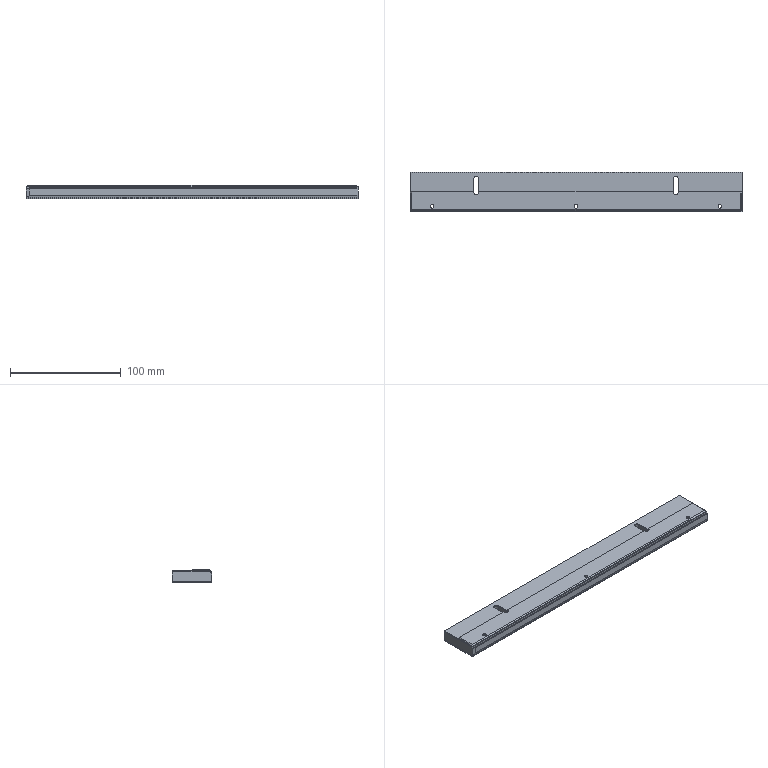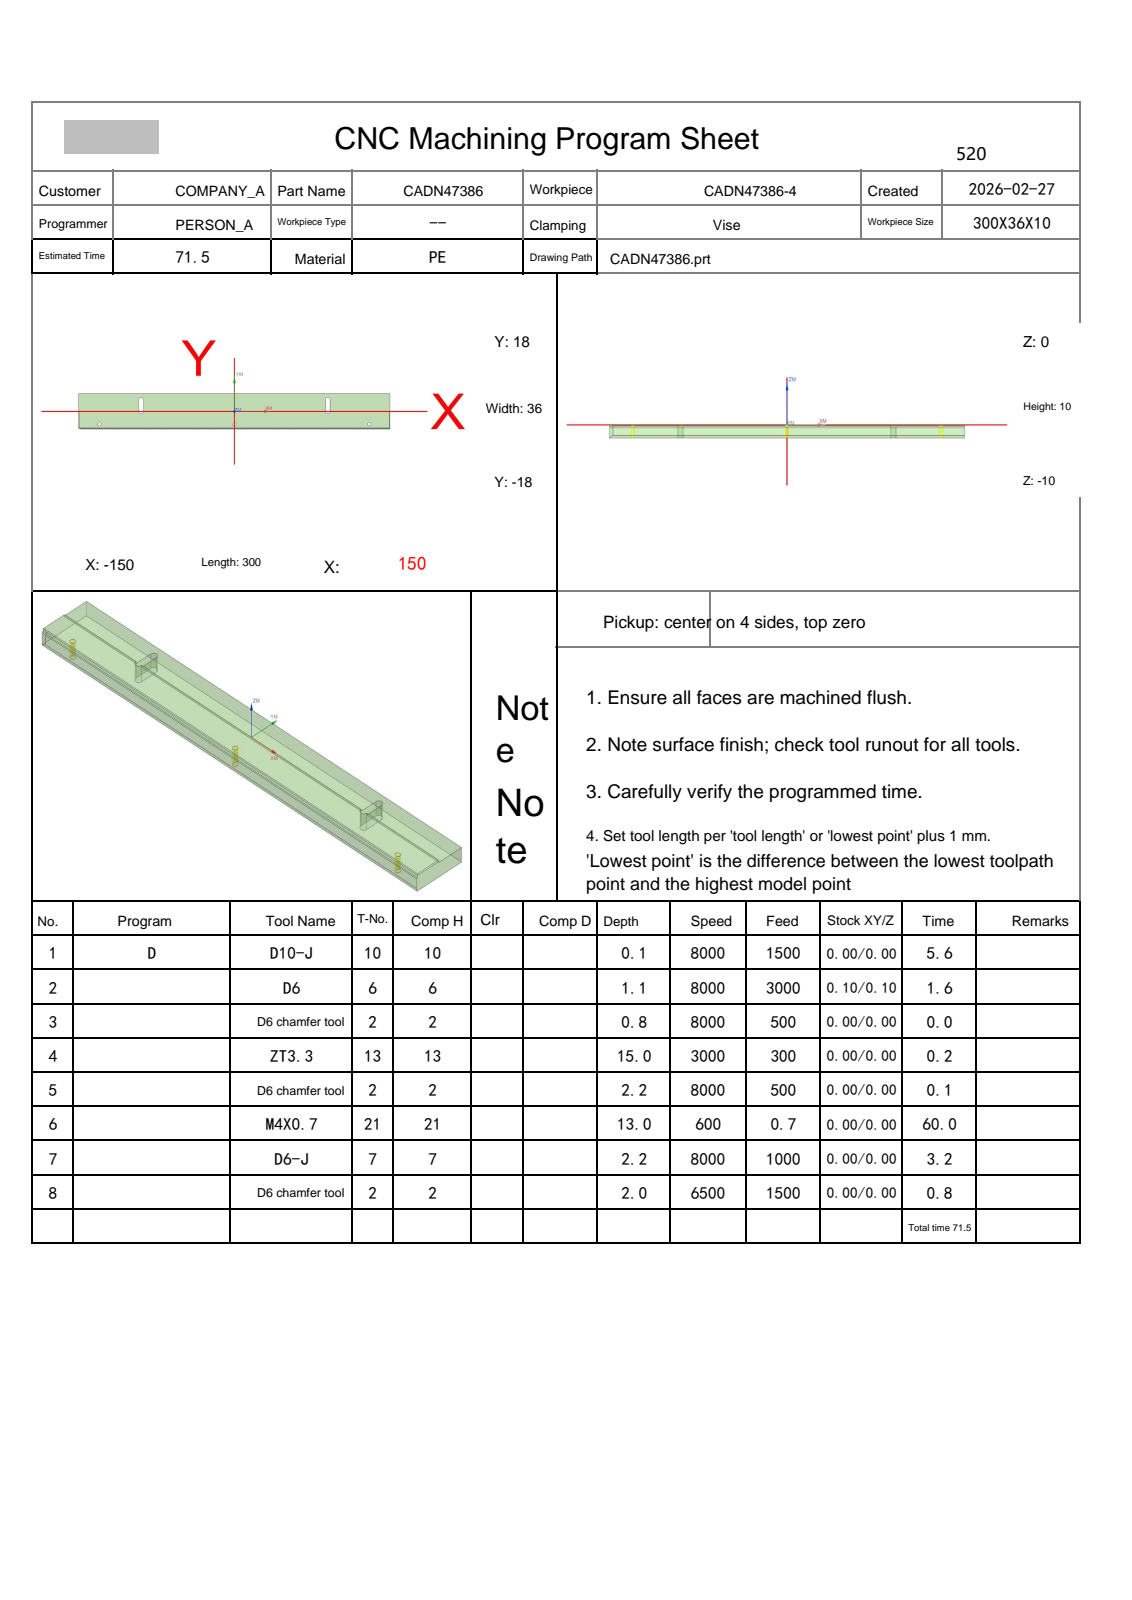NC program | NX | posted by the shop | part box 300 x 36 x 12 mm
Whole program:
%
O0001
(Machine time: 128.86 MIN)
(===Total Tool:6===)
(T10=D10-J  D=10.  R=0.   D-  H10 Z=0.    )
(T6=D6      D=6.   R=0.   D-  H06 Z=-1.1  )
(T2=D6 chamfer tool   D=6.   R=0.   D-  H02 Z=-2.17 )
(T13=ZT3.3  D=3.3  DR_a=118 D-  H13 Z=-15.  )
(T21=M4X0.7 D=3.3  DR_a=180 D-  H21 Z=-13.  )
(T7=D6-J    D=6.   R=0.   D7  H07 Z=-2.2  )
G80 G90 G17 G49 G40
G91 G28 Z0
M01
N1 T10 M06
(D10-J  D=10. R=0. H=10 ce=0.00 di=0.10)
G00 G90 G54 X-160. Y8.111 M03 S4500
G43 H10 Z30.
M08
Z2.55
G01 Z.55 F1500.
X-155. Y13.111
X-145.111 Y23.
X-135.222
X-155. Y3.222
Y-6.667
X-125.333 Y23.
X-115.444
X-155. Y-16.556
Y-23.
X-151.556
X-105.556 Y23.
X-95.667
X-141.667 Y-23.
X-131.778
X-85.778 Y23.
X-75.889
X-121.889 Y-23.
X-112.
X-66. Y23.
X-56.111
X-102.111 Y-23.
X-92.222
X-46.222 Y23.
X-36.333
X-82.333 Y-23.
X-72.444
X-26.444 Y23.
X-16.556
X-62.556 Y-23.
X-52.667
X-6.667 Y23.
X3.222
X-42.778 Y-23.
X-32.889
X13.111 Y23.
X23.
X-23. Y-23.
X-13.111
X32.889 Y23.
X42.778
X-3.222 Y-23.
X6.667
X52.667 Y23.
X62.556
X16.556 Y-23.
X26.444
X72.444 Y23.
X82.333
X36.333 Y-23.
X46.222
X92.222 Y23.
X102.111
X56.111 Y-23.
X66.
X112. Y23.
X121.889
X75.889 Y-23.
X85.778
X131.778 Y23.
X141.667
X95.667 Y-23.
X105.556
X151.556 Y23.
X155.
Y16.556
X115.444 Y-23.
X125.333
X155. Y6.667
Y-3.222
X135.222 Y-23.
X145.111
X155. Y-13.111
X160. Y-8.111
Z2.55
G00 Z4.
X-160. Y8.111
Z2.1
G01 Z.1
X-155. Y13.111
X-145.111 Y23.
X-135.222
X-155. Y3.222
Y-6.667
X-125.333 Y23.
X-115.444
X-155. Y-16.556
Y-23.
X-151.556
X-105.556 Y23.
X-95.667
X-141.667 Y-23.
X-131.778
X-85.778 Y23.
X-75.889
X-121.889 Y-23.
X-112.
X-66. Y23.
X-56.111
X-102.111 Y-23.
X-92.222
X-46.222 Y23.
X-36.333
X-82.333 Y-23.
X-72.444
X-26.444 Y23.
X-16.556
X-62.556 Y-23.
X-52.667
X-6.667 Y23.
X3.222
X-42.778 Y-23.
X-32.889
X13.111 Y23.
X23.
X-23. Y-23.
X-13.111
X32.889 Y23.
X42.778
X-3.222 Y-23.
X6.667
X52.667 Y23.
X62.556
X16.556 Y-23.
X26.444
X72.444 Y23.
X82.333
X36.333 Y-23.
X46.222
X92.222 Y23.
X102.111
X56.111 Y-23.
X66.
X112. Y23.
X121.889
X75.889 Y-23.
X85.778
X131.778 Y23.
X141.667
X95.667 Y-23.
X105.556
X151.556 Y23.
X155.
Y16.556
X115.444 Y-23.
X125.333
X155. Y6.667
Y-3.222
X135.222 Y-23.
X145.111
X155. Y-13.111
X160. Y-8.111
Z2.1
G00 Z30.
G00 G90 X133.111 Y35. M03 S8000
Z30.
Z2.
G01 Z0.0 F1000.
X145.111 Y23.
X155. Y13.111
Y3.222
X135.222 Y23.
X125.333
X155. Y-6.667
Y-16.556
X115.444 Y23.
X105.556
X151.556 Y-23.
X141.667
X95.667 Y23.
X85.778
X131.778 Y-23.
X121.889
X75.889 Y23.
X66.
X112. Y-23.
X102.111
X56.111 Y23.
X46.222
X92.222 Y-23.
X82.333
X36.333 Y23.
X26.444
X72.444 Y-23.
X62.556
X16.556 Y23.
X6.667
X52.667 Y-23.
X42.778
X-3.222 Y23.
X-13.111
X32.889 Y-23.
X23.
X-23. Y23.
X-32.889
X13.111 Y-23.
X3.222
X-42.778 Y23.
X-52.667
X-6.667 Y-23.
X-16.556
X-62.556 Y23.
X-72.444
X-26.444 Y-23.
X-36.333
X-82.333 Y23.
X-92.222
X-46.222 Y-23.
X-56.111
X-102.111 Y23.
X-112.
X-66. Y-23.
X-75.889
X-121.889 Y23.
X-131.778
X-85.778 Y-23.
X-95.667
X-141.667 Y23.
X-151.556
X-105.556 Y-23.
X-115.444
X-155. Y16.556
Y6.667
X-125.333 Y-23.
X-135.222
X-155. Y-3.222
Y-13.111
X-145.111 Y-23.
X-133.111 Y-35.
Z2.
G00 Z30.
G91 G28 Z0.0
M05
M09
G91 G28 Z0.0
M01
N2 T06 M06
(D6  D=6. R=0. H=06 ce=0.10 di=0.10)
G00 G90 G54 X-156. Y19.6 M03 S8000
G43 H06 Z11.
M08
Z1.133
G01 Z-.367 F3000.
X-152.94
X152.4
G02 X152.94 Y19.06 I0.0 J-.54
G01 Y17.2
G02 X152.34 Y16.6 I-.6 J0.0
G01 X-152.341
G03 X-152.94 Y16.001 I.001 J-.6
G01 Y12.699
G03 X-152.341 Y12.1 I.6 J.001
G01 X152.341
G02 X152.94 Y11.501 I-.001 J-.6
G01 Y8.199
G02 X152.341 Y7.6 I-.6 J.001
G01 X-152.427
G03 X-153.019 Y7.093 I.001 J-.6
G01 X-153.533 Y3.792
X-153.54 Y3.7
G03 X-152.94 Y3.1 I.6 J0.0
G01 X152.94
X156.
Z1.133
G00 X-156. Y19.6
Z.767
G01 Z-.733
X-152.94
X152.4
G02 X152.94 Y19.06 I0.0 J-.54
G01 Y17.2
G02 X152.34 Y16.6 I-.6 J0.0
G01 X-152.341
G03 X-152.94 Y16.001 I.001 J-.6
G01 Y12.699
G03 X-152.341 Y12.1 I.6 J.001
G01 X152.341
G02 X152.94 Y11.501 I-.001 J-.6
G01 Y8.199
G02 X152.341 Y7.6 I-.6 J.001
G01 X-152.427
G03 X-153.019 Y7.093 I.001 J-.6
G01 X-153.533 Y3.792
X-153.54 Y3.7
G03 X-152.94 Y3.1 I.6 J0.0
G01 X152.94
X156.1
Z.767
G00 X-156. Y19.6
Z.4
G01 Z-1.1
X-152.94
X152.4
G02 X152.94 Y19.06 I0.0 J-.54
G01 Y17.2
G02 X152.34 Y16.6 I-.6 J0.0
G01 X-152.341
G03 X-152.94 Y16.001 I.001 J-.6
G01 Y12.699
G03 X-152.341 Y12.1 I.6 J.001
G01 X152.341
G02 X152.94 Y11.501 I-.001 J-.6
G01 Y8.199
G02 X152.341 Y7.6 I-.6 J.001
G01 X-152.427
G03 X-153.019 Y7.093 I.001 J-.6
G01 X-153.533 Y3.792
X-153.54 Y3.7
G03 X-152.94 Y3.1 I.6 J0.0
G01 X152.94
X156.1
Z.4
G00 Z11.
G91 G28 Z0.0
M05
M09
G91 G28 Z0.0
M01
N3 T02 M06
(D6 chamfer tool  D=6. R=0. H=02 ce=0.00 di=0.10)
G00 G90 G54 X130. Y-13. M03 S8000
G43 H02 Z30.
M08
G98 G81 X130. Y-13. Z-.8 R1. F500.
X0.0
X-130.
G80
G00 Z30.
G91 G28 Z0.0
M05
M09
G91 G28 Z0.0
M01
N4 T13 M06
(ZT3.3 D=3.3 DR_a=118 H=13)
G00 G90 G54 X130. Y-13. M03 S3000
G43 H13 Z30.
M08
G98 G83 X130. Y-13. Z-15. R1. F300. Q2.
X0.0
X-130.
G80
G00 Z30.
G91 G28 Z0.0
M05
M09
G91 G28 Z0.0
M01
N5 T02 M06
(D6 chamfer tool  D=6. R=0. H=02 ce=0.00 di=0.10)
G00 G90 G54 X130. Y-13. M03 S8000
G43 H02 Z30.
M08
G98 G81 X130. Y-13. Z-2.171 R3. F500.
X0.0
X-130.
G80
G00 Z30.
G91 G28 Z0.0
M05
M09
G91 G28 Z0.0
M01
N6 T21 M06
(M4X0.7 D=3.3 DR_a=180 H=21)
G00 G90 G54 X130. Y-13. M03 S600
G43 H21 Z30.
M08
G95
G98 G84 X130. Y-13. Z-13. R1. F.7 Q4.
X0.0
X-130.
G80
G94
G00 Z30.
G91 G28 Z0.0
M05
M09
G91 G28 Z0.0
M01
N7 T07 M06
(D6-J  D=6. R=0. H=07 ce=0.40 di=0.00)
G00 G90 G54 X-1.2 Y22.2 M03 S8000
G43 H07 Z11.
M08
Z.3
G01 Z-1.2 F1000.
Y19.8
G03 X0.0 Y18.6 I1.2 J0.0
G01 X150.004
G02 X150.6 Y18.004 I-.004 J-.6
G01 Y3.996
G02 X150.004 Y3.4 I-.6 J.004
G01 X-150.004
G02 X-150.6 Y3.996 I.004 J.6
G01 Y18.004
G02 X-150.004 Y18.6 I.6 J-.004
G01 X1.252
G02 X1.675 Y18.425 I-.001 J-.6
G01 X4.325 Y15.775
G03 X4.748 Y15.6 I.424 J.425
G01 X147.004
G02 X147.6 Y15.004 I-.004 J-.6
G01 Y6.996
G02 X147.004 Y6.4 I-.6 J.004
G01 X-147.004
G02 X-147.6 Y6.996 I.004 J.6
G01 Y15.004
G02 X-147.004 Y15.6 I.6 J-.004
G01 X1.252
G02 X1.675 Y15.425 I-.001 J-.6
G01 X4.325 Y12.775
G03 X4.748 Y12.6 I.424 J.425
G01 X144.004
G02 X144.6 Y12.004 I-.004 J-.6
G01 Y9.996
G02 X144.004 Y9.4 I-.6 J.004
G01 X88.85
X-144.004
G02 X-144.6 Y9.996 I.004 J.6
G01 Y12.004
G02 X-144.004 Y12.6 I.6 J-.004
G01 X3.
X4.
G03 X5.2 Y13.8 I0.0 J1.2
G01 Z.3
G00 Z11.
G00 G90 X-154.2 Y4.399 M03 S8000
Z11.
Z-.2
G01 Z-1.2 F1000.
G41 D07
Y4.199
G03 X-153. Y3. I1.2 J.001
G01 X153.
G03 X154.2 Y4.199 I0.0 J1.2
G01 G40 Y4.399
Z-.2
G00 Z11.
G00 G90 X153.916 Y-21.226 M03 S8000
Z11.
Z.719
G01 Z-.781 F1000.
G41 D07
X153.9 Y-21.027
G03 X153.003 Y-20.2 I-.897 J-.073
G01 X-147.248
X-153.455 Y-19.165
X-153.603 Y-19.153
G03 X-153.9 Y-19.204 I0.0 J-.9
G01 G40 X-154.089 Y-19.27
Z.719
G00 Z11.
X153.916 Y-21.226
Z.01
G01 Z-1.49
G41 D07
X153.9 Y-21.027
G03 X153.003 Y-20.2 I-.897 J-.073
G01 X-147.248
X-153.455 Y-19.165
X-153.603 Y-19.153
G03 X-153.9 Y-19.204 I0.0 J-.9
G01 G40 X-154.089 Y-19.27
Z.01
G00 Z11.
X153.916 Y-21.226
Z-.7
G01 Z-2.2
G41 D07
X153.9 Y-21.027
G03 X153.003 Y-20.2 I-.897 J-.073
G01 X-147.248
X-153.455 Y-19.165
X-153.603 Y-19.153
G03 X-153.9 Y-19.204 I0.0 J-.9
G01 G40 X-154.089 Y-19.27
Z-.7
G00 Z11.
G91 G28 Z0.0
M05
M09
G91 G28 Z0.0
M01
N8 T02 M06
(D6 chamfer tool  D=6. R=0. H=02 ce=0.00 di=0.00)
G00 G90 G54 X-149.769 Y.528 M03 S6500
G43 H02 Z30.
M08
Z3.2
G01 Z-.8 F1500.
X-149.685 Y.571
X-149.5 Y.6
X-92.25
G02 X-91.65 Y0.0 I0.0 J-.6
G01 Y-.2
G03 X-90. Y-1.85 I1.65 J0.0
X-88.35 Y-.2 I0.0 J1.65
G01 Y0.0
G02 X-87.75 Y.6 I.6 J0.0
G01 X87.75
G02 X88.35 Y0.0 I0.0 J-.6
G01 Y-.2
G03 X90. Y-1.85 I1.65 J0.0
X91.65 Y-.2 I0.0 J1.65
G01 Y0.0
G02 X92.25 Y.6 I.6 J0.0
G01 X149.5
X149.685 Y.571
X149.769 Y.528
Z3.2
G00 Z10.
X130.847 Y-13.412
Z.728
G01 Z-.8
G03 X131.007 Y-13.103 I-1.687 J1.075
G01 X131.031 Y-13.054
X131.021 Y-13.
G03 X130. Y-11.979 I-1.021 J0.0
X128.979 Y-13. I0.0 J-1.021
X130. Y-14.021 I1.021 J0.0
X131.021 Y-13. I0.0 J1.021
G01 X131.031 Y-12.946
X131.007 Y-12.897
G03 X130.847 Y-12.588 I-1.848 J-.765
G01 Z.728
G00 Z10.
X.847 Y-13.412
Z.728
G01 Z-.8
G03 X1.007 Y-13.103 I-1.687 J1.075
G01 X1.031 Y-13.054
X1.021 Y-13.
G03 X0.0 Y-11.979 I-1.021 J0.0
X-1.021 Y-13. I0.0 J-1.021
X0.0 Y-14.021 I1.021 J0.0
X1.021 Y-13. I0.0 J1.021
G01 X1.031 Y-12.946
X1.007 Y-12.897
G03 X.847 Y-12.588 I-1.848 J-.765
G01 Z.728
G00 Z10.
X-129.153 Y-13.412
Z.728
G01 Z-.8
G03 X-128.993 Y-13.103 I-1.687 J1.075
G01 X-128.969 Y-13.054
X-128.979 Y-13.
G03 X-130. Y-11.979 I-1.021 J0.0
X-131.021 Y-13. I0.0 J-1.021
X-130. Y-14.021 I1.021 J0.0
X-128.979 Y-13. I0.0 J1.021
G01 X-128.969 Y-12.946
X-128.993 Y-12.897
G03 X-129.153 Y-12.588 I-1.848 J-.765
G01 Z.728
G00 Z10.
X-88.35 Y1.89
Z2.
G01 Z-2.
Y11.8
G03 X-90. Y13.45 I-1.65 J0.0
X-91.65 Y11.8 I0.0 J-1.65
G01 Y1.89
Z2.
G00 Z10.
X91.65
Z2.
G01 Z-2.
Y11.8
G03 X90. Y13.45 I-1.65 J0.0
X88.35 Y11.8 I0.0 J-1.65
G01 Y1.89
Z2.
G00 Z10.
X-150.6 Y1.652
Z2.
G01 Z-2.
Y18.
G02 X-150. Y18.6 I.6 J0.0
G01 X150.
G02 X150.6 Y18. I0.0 J-.6
G01 Y1.652
Z2.
G00 Z30.
G00 G90 X151.9 Y3.963 M03 S6500
Z30.
Z.3
G01 Z-1.2 F1500.
G03 X150.7 Y2.763 I0.0 J-1.2
G01 Y-17.9
X-150.7
Y2.763
G03 X-151.9 Y3.963 I-1.2 J0.0
G01 Z.3
G00 Z30.
M05
M09
G91 G28 Z0.0
G91 G28 Y0.0
M30
%